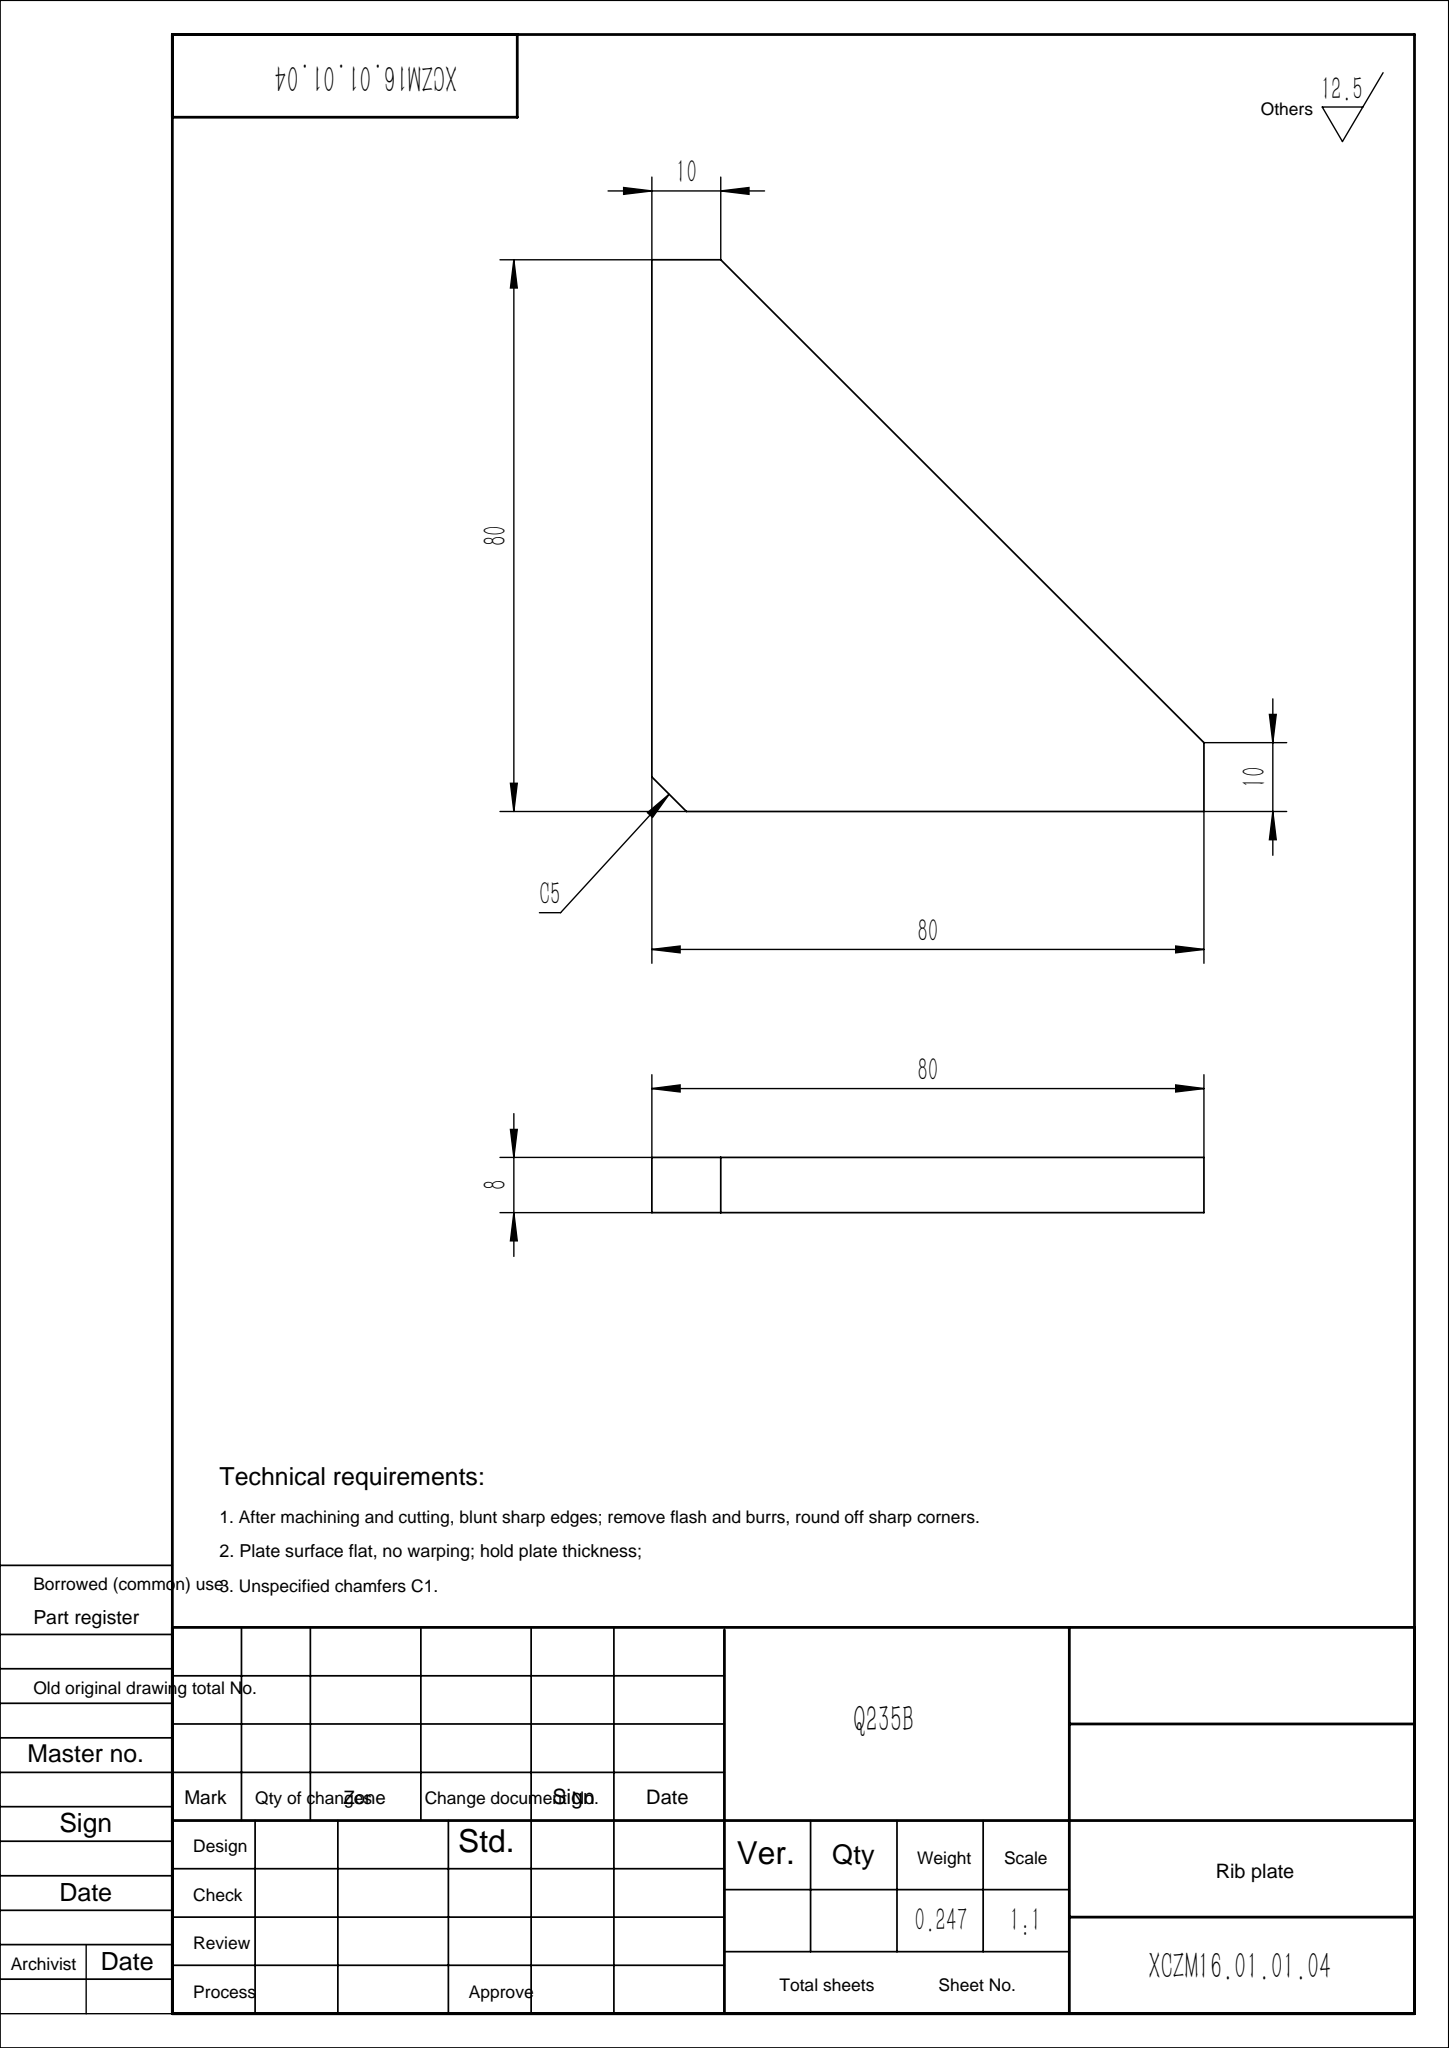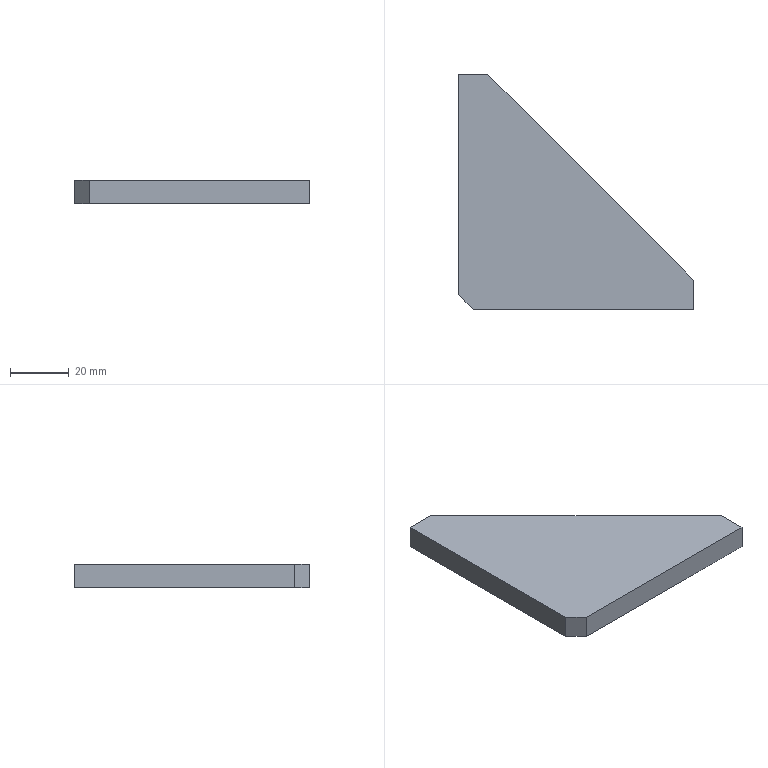Part | SolidWorks | features Chamfer 1, Extrusion 1 | 1 solid | 8 faces | box 80 x 80 x 8 mm | volume 31500 mm3 | plane 8
STEP:
#1=CARTESIAN_POINT('',(10.,80.,0.));
#2=VERTEX_POINT('',#1);
#3=CARTESIAN_POINT('',(0.,80.,0.));
#4=VERTEX_POINT('',#3);
#5=CARTESIAN_POINT('',(10.,80.,0.));
#6=DIRECTION('',(-1.,0.,0.));
#7=VECTOR('',#6,1000.);
#8=LINE('',#5,#7);
#9=EDGE_CURVE('',#2,#4,#8,.T.);
#10=ORIENTED_EDGE('',*,*,#9,.T.);
#11=CARTESIAN_POINT('',(0.,80.,8.));
#12=VERTEX_POINT('',#11);
#13=CARTESIAN_POINT('',(0.,80.,8.));
#14=DIRECTION('',(0.,0.,-1.));
#15=VECTOR('',#14,1000.);
#16=LINE('',#13,#15);
#17=EDGE_CURVE('',#12,#4,#16,.T.);
#18=ORIENTED_EDGE('',*,*,#17,.F.);
#19=CARTESIAN_POINT('',(10.,80.,8.));
#20=VERTEX_POINT('',#19);
#21=CARTESIAN_POINT('',(10.,80.,8.));
#22=DIRECTION('',(-1.,0.,0.));
#23=VECTOR('',#22,1000.);
#24=LINE('',#21,#23);
#25=EDGE_CURVE('',#20,#12,#24,.T.);
#26=ORIENTED_EDGE('',*,*,#25,.F.);
#27=CARTESIAN_POINT('',(10.,80.,8.));
#28=DIRECTION('',(0.,0.,-1.));
#29=VECTOR('',#28,1000.);
#30=LINE('',#27,#29);
#31=EDGE_CURVE('',#20,#2,#30,.T.);
#32=ORIENTED_EDGE('',*,*,#31,.T.);
#33=EDGE_LOOP('',(#10,#18,#26,#32));
#34=FACE_OUTER_BOUND('',#33,.T.);
#35=CARTESIAN_POINT('',(10.,80.,8.));
#36=DIRECTION('',(0.,-1.,0.));
#37=DIRECTION('',(0.,0.,-1.));
#38=AXIS2_PLACEMENT_3D('',#35,#36,#37);
#39=PLANE('',#38);
#40=ADVANCED_FACE('',(#34),#39,.F.);
#41=CARTESIAN_POINT('',(0.,5.,0.));
#42=VERTEX_POINT('',#41);
#43=CARTESIAN_POINT('',(0.,80.,0.));
#44=DIRECTION('',(0.,-1.,0.));
#45=VECTOR('',#44,1000.);
#46=LINE('',#43,#45);
#47=EDGE_CURVE('',#4,#42,#46,.T.);
#48=ORIENTED_EDGE('',*,*,#47,.T.);
#49=CARTESIAN_POINT('',(0.,5.,8.));
#50=VERTEX_POINT('',#49);
#51=CARTESIAN_POINT('',(0.,5.,8.));
#52=DIRECTION('',(0.,0.,1.));
#53=VECTOR('',#52,1000.);
#54=LINE('',#51,#53);
#55=EDGE_CURVE('',#42,#50,#54,.T.);
#56=ORIENTED_EDGE('',*,*,#55,.T.);
#57=CARTESIAN_POINT('',(0.,80.,8.));
#58=DIRECTION('',(0.,-1.,0.));
#59=VECTOR('',#58,1000.);
#60=LINE('',#57,#59);
#61=EDGE_CURVE('',#12,#50,#60,.T.);
#62=ORIENTED_EDGE('',*,*,#61,.F.);
#63=ORIENTED_EDGE('',*,*,#17,.T.);
#64=EDGE_LOOP('',(#48,#56,#62,#63));
#65=FACE_OUTER_BOUND('',#64,.T.);
#66=CARTESIAN_POINT('',(0.,80.,8.));
#67=DIRECTION('',(1.,0.,0.));
#68=DIRECTION('',(0.,1.,0.));
#69=AXIS2_PLACEMENT_3D('',#66,#67,#68);
#70=PLANE('',#69);
#71=ADVANCED_FACE('',(#65),#70,.F.);
#72=CARTESIAN_POINT('',(5.,0.,8.));
#73=VERTEX_POINT('',#72);
#74=CARTESIAN_POINT('',(80.,0.,8.));
#75=VERTEX_POINT('',#74);
#76=CARTESIAN_POINT('',(0.,0.,8.));
#77=DIRECTION('',(1.,0.,0.));
#78=VECTOR('',#77,1000.);
#79=LINE('',#76,#78);
#80=EDGE_CURVE('',#73,#75,#79,.T.);
#81=ORIENTED_EDGE('',*,*,#80,.F.);
#82=CARTESIAN_POINT('',(5.,0.,0.));
#83=VERTEX_POINT('',#82);
#84=CARTESIAN_POINT('',(5.,0.,8.));
#85=DIRECTION('',(0.,0.,-1.));
#86=VECTOR('',#85,1000.);
#87=LINE('',#84,#86);
#88=EDGE_CURVE('',#73,#83,#87,.T.);
#89=ORIENTED_EDGE('',*,*,#88,.T.);
#90=CARTESIAN_POINT('',(80.,0.,0.));
#91=VERTEX_POINT('',#90);
#92=CARTESIAN_POINT('',(0.,0.,0.));
#93=DIRECTION('',(1.,0.,0.));
#94=VECTOR('',#93,1000.);
#95=LINE('',#92,#94);
#96=EDGE_CURVE('',#83,#91,#95,.T.);
#97=ORIENTED_EDGE('',*,*,#96,.T.);
#98=CARTESIAN_POINT('',(80.,0.,8.));
#99=DIRECTION('',(0.,0.,-1.));
#100=VECTOR('',#99,1000.);
#101=LINE('',#98,#100);
#102=EDGE_CURVE('',#75,#91,#101,.T.);
#103=ORIENTED_EDGE('',*,*,#102,.F.);
#104=EDGE_LOOP('',(#81,#89,#97,#103));
#105=FACE_OUTER_BOUND('',#104,.T.);
#106=CARTESIAN_POINT('',(0.,0.,8.));
#107=DIRECTION('',(0.,1.,0.));
#108=DIRECTION('',(0.,0.,1.));
#109=AXIS2_PLACEMENT_3D('',#106,#107,#108);
#110=PLANE('',#109);
#111=ADVANCED_FACE('',(#105),#110,.F.);
#112=CARTESIAN_POINT('',(80.,10.,0.));
#113=VERTEX_POINT('',#112);
#114=CARTESIAN_POINT('',(80.,0.,0.));
#115=DIRECTION('',(0.,1.,0.));
#116=VECTOR('',#115,1000.);
#117=LINE('',#114,#116);
#118=EDGE_CURVE('',#91,#113,#117,.T.);
#119=ORIENTED_EDGE('',*,*,#118,.T.);
#120=CARTESIAN_POINT('',(80.,10.,8.));
#121=VERTEX_POINT('',#120);
#122=CARTESIAN_POINT('',(80.,10.,8.));
#123=DIRECTION('',(0.,0.,-1.));
#124=VECTOR('',#123,1000.);
#125=LINE('',#122,#124);
#126=EDGE_CURVE('',#121,#113,#125,.T.);
#127=ORIENTED_EDGE('',*,*,#126,.F.);
#128=CARTESIAN_POINT('',(80.,0.,8.));
#129=DIRECTION('',(0.,1.,0.));
#130=VECTOR('',#129,1000.);
#131=LINE('',#128,#130);
#132=EDGE_CURVE('',#75,#121,#131,.T.);
#133=ORIENTED_EDGE('',*,*,#132,.F.);
#134=ORIENTED_EDGE('',*,*,#102,.T.);
#135=EDGE_LOOP('',(#119,#127,#133,#134));
#136=FACE_OUTER_BOUND('',#135,.T.);
#137=CARTESIAN_POINT('',(80.,0.,8.));
#138=DIRECTION('',(-1.,0.,0.));
#139=DIRECTION('',(0.,0.,1.));
#140=AXIS2_PLACEMENT_3D('',#137,#138,#139);
#141=PLANE('',#140);
#142=ADVANCED_FACE('',(#136),#141,.F.);
#143=CARTESIAN_POINT('',(80.,10.,0.));
#144=DIRECTION('',(-0.7071,0.7071,0.));
#145=VECTOR('',#144,1000.);
#146=LINE('',#143,#145);
#147=EDGE_CURVE('',#113,#2,#146,.T.);
#148=ORIENTED_EDGE('',*,*,#147,.T.);
#149=ORIENTED_EDGE('',*,*,#31,.F.);
#150=CARTESIAN_POINT('',(80.,10.,8.));
#151=DIRECTION('',(-0.7071,0.7071,0.));
#152=VECTOR('',#151,1000.);
#153=LINE('',#150,#152);
#154=EDGE_CURVE('',#121,#20,#153,.T.);
#155=ORIENTED_EDGE('',*,*,#154,.F.);
#156=ORIENTED_EDGE('',*,*,#126,.T.);
#157=EDGE_LOOP('',(#148,#149,#155,#156));
#158=FACE_OUTER_BOUND('',#157,.T.);
#159=CARTESIAN_POINT('',(80.,10.,8.));
#160=DIRECTION('',(-0.7071,-0.7071,0.));
#161=DIRECTION('',(0.7071,-0.7071,0.));
#162=AXIS2_PLACEMENT_3D('',#159,#160,#161);
#163=PLANE('',#162);
#164=ADVANCED_FACE('',(#158),#163,.F.);
#165=ORIENTED_EDGE('',*,*,#61,.T.);
#166=CARTESIAN_POINT('',(2.5,2.5,8.));
#167=DIRECTION('',(0.7071,-0.7071,0.));
#168=VECTOR('',#167,1000.);
#169=LINE('',#166,#168);
#170=EDGE_CURVE('',#50,#73,#169,.T.);
#171=ORIENTED_EDGE('',*,*,#170,.T.);
#172=ORIENTED_EDGE('',*,*,#80,.T.);
#173=ORIENTED_EDGE('',*,*,#132,.T.);
#174=ORIENTED_EDGE('',*,*,#154,.T.);
#175=ORIENTED_EDGE('',*,*,#25,.T.);
#176=EDGE_LOOP('',(#165,#171,#172,#173,#174,#175));
#177=FACE_OUTER_BOUND('',#176,.T.);
#178=CARTESIAN_POINT('',(0.,0.,8.));
#179=DIRECTION('',(0.,0.,1.));
#180=DIRECTION('',(1.,0.,0.));
#181=AXIS2_PLACEMENT_3D('',#178,#179,#180);
#182=PLANE('',#181);
#183=ADVANCED_FACE('',(#177),#182,.T.);
#184=ORIENTED_EDGE('',*,*,#96,.F.);
#185=CARTESIAN_POINT('',(5.,0.,0.));
#186=DIRECTION('',(-0.7071,0.7071,0.));
#187=VECTOR('',#186,1000.);
#188=LINE('',#185,#187);
#189=EDGE_CURVE('',#83,#42,#188,.T.);
#190=ORIENTED_EDGE('',*,*,#189,.T.);
#191=ORIENTED_EDGE('',*,*,#47,.F.);
#192=ORIENTED_EDGE('',*,*,#9,.F.);
#193=ORIENTED_EDGE('',*,*,#147,.F.);
#194=ORIENTED_EDGE('',*,*,#118,.F.);
#195=EDGE_LOOP('',(#184,#190,#191,#192,#193,#194));
#196=FACE_OUTER_BOUND('',#195,.T.);
#197=CARTESIAN_POINT('',(0.,0.,0.));
#198=DIRECTION('',(0.,0.,1.));
#199=DIRECTION('',(1.,0.,0.));
#200=AXIS2_PLACEMENT_3D('',#197,#198,#199);
#201=PLANE('',#200);
#202=ADVANCED_FACE('',(#196),#201,.F.);
#203=ORIENTED_EDGE('',*,*,#170,.F.);
#204=ORIENTED_EDGE('',*,*,#55,.F.);
#205=ORIENTED_EDGE('',*,*,#189,.F.);
#206=ORIENTED_EDGE('',*,*,#88,.F.);
#207=EDGE_LOOP('',(#203,#204,#205,#206));
#208=FACE_OUTER_BOUND('',#207,.T.);
#209=CARTESIAN_POINT('',(5.,0.,8.));
#210=DIRECTION('',(0.7071,0.7071,0.));
#211=DIRECTION('',(0.,0.,-1.));
#212=AXIS2_PLACEMENT_3D('',#209,#210,#211);
#213=PLANE('',#212);
#214=ADVANCED_FACE('',(#208),#213,.F.);
#215=CLOSED_SHELL('',(#40,#71,#111,#142,#164,#183,#202,#214));
#216=MANIFOLD_SOLID_BREP('',#215);
#217=CARTESIAN_POINT('',(0.,0.,0.));
#218=DIRECTION('',(0.,0.,1.));
#219=DIRECTION('',(1.,0.,0.));
#220=AXIS2_PLACEMENT_3D('',#217,#218,#219);
#221=(LENGTH_UNIT()NAMED_UNIT(*)SI_UNIT(.MILLI.,.METRE.));
#222=UNCERTAINTY_MEASURE_WITH_UNIT(LENGTH_MEASURE(0.00001),#221,'','');
#223=(NAMED_UNIT(*)PLANE_ANGLE_UNIT()SI_UNIT($,.RADIAN.));
#224=(NAMED_UNIT(*)SI_UNIT($,.STERADIAN.)SOLID_ANGLE_UNIT());
#225=(GEOMETRIC_REPRESENTATION_CONTEXT(3)GLOBAL_UNCERTAINTY_ASSIGNED_CONTEXT((#222))GLOBAL_UNIT_ASSIGNED_CONTEXT((#221,#223,#224))REPRESENTATION_CONTEXT('',''));
#226=ADVANCED_BREP_SHAPE_REPRESENTATION('',(#216,#220),#225);